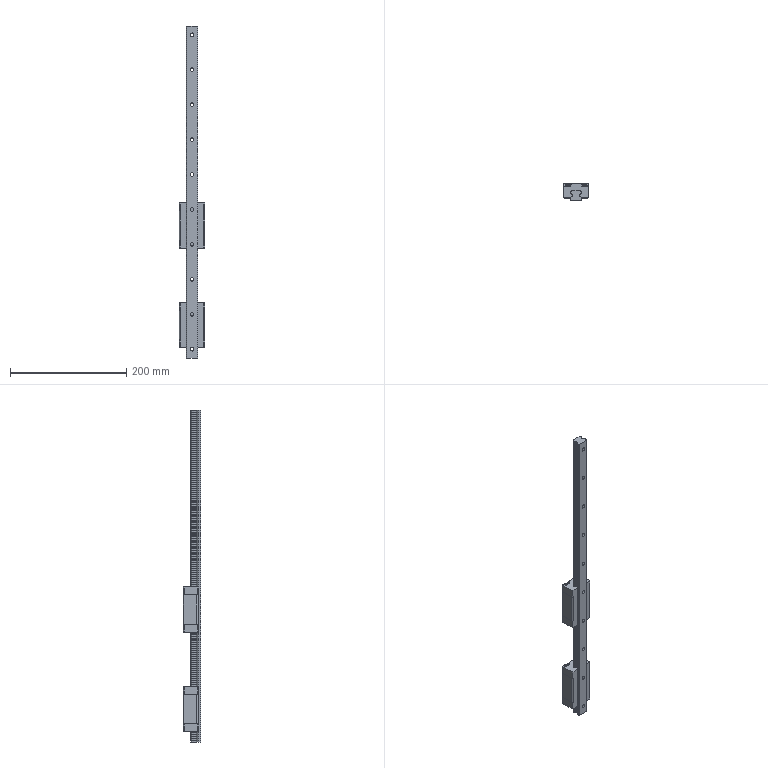Part | SolidWorks | 3 solids | 848 faces | box 44 x 30 x 570 mm | volume 296416 mm3 | plane 602 | cylinder 126 | spline 120 | commonest cylinder face diameters 1 x36 2 x22 6 x20 9.5 x20 5 x16 4.06 x12